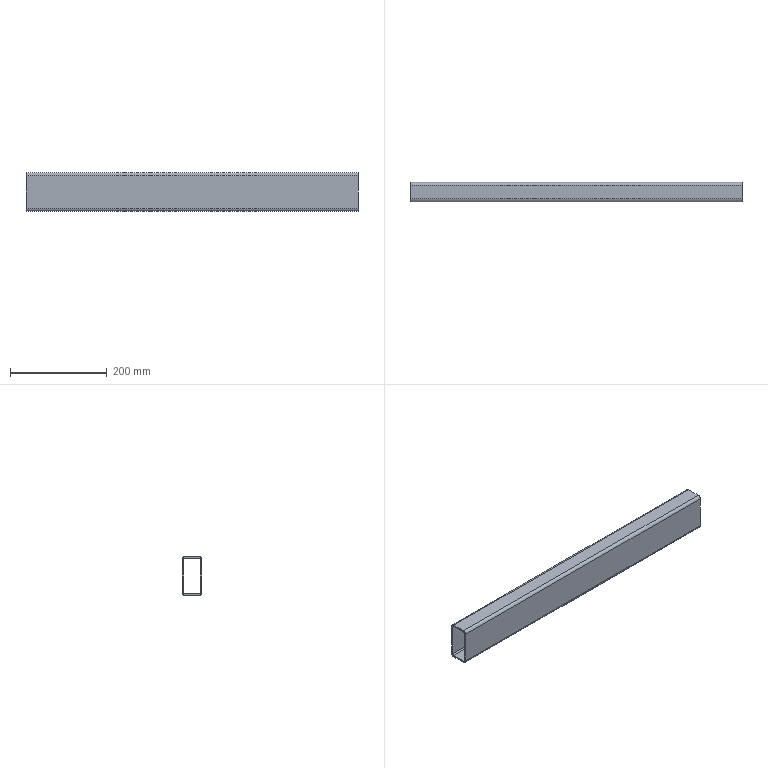Part | 1 solid | 34 faces | box 686 x 40 x 80 mm | volume 451963 mm3 | cylinder 24 | plane 10 | commonest cylinder face diameters 8.5 x16 6 x4 12 x4
STEP:
#1=CARTESIAN_POINT('',(478.,17.,13.25));
#2=VERTEX_POINT('',#1);
#3=CARTESIAN_POINT('',(478.,17.,21.75));
#4=VERTEX_POINT('',#3);
#5=CARTESIAN_POINT('',(478.,17.,17.5));
#6=DIRECTION('',(0.,1.,0.));
#7=DIRECTION('',(0.,0.,-1.));
#8=AXIS2_PLACEMENT_3D('',#5,#6,#7);
#9=CIRCLE('',#8,4.25);
#10=EDGE_CURVE('',#2,#4,#9,.T.);
#11=ORIENTED_EDGE('',*,*,#10,.F.);
#12=CARTESIAN_POINT('',(478.,20.,13.25));
#13=VERTEX_POINT('',#12);
#14=CARTESIAN_POINT('',(478.,-20.001,13.25));
#15=DIRECTION('',(0.,1.,0.));
#16=VECTOR('',#15,1000.);
#17=LINE('',#14,#16);
#18=EDGE_CURVE('',#2,#13,#17,.T.);
#19=ORIENTED_EDGE('',*,*,#18,.T.);
#20=CARTESIAN_POINT('',(478.,20.,21.75));
#21=VERTEX_POINT('',#20);
#22=CARTESIAN_POINT('',(478.,20.,17.5));
#23=DIRECTION('',(0.,1.,0.));
#24=DIRECTION('',(0.,0.,-1.));
#25=AXIS2_PLACEMENT_3D('',#22,#23,#24);
#26=CIRCLE('',#25,4.25);
#27=EDGE_CURVE('',#13,#21,#26,.T.);
#28=ORIENTED_EDGE('',*,*,#27,.T.);
#29=CARTESIAN_POINT('',(478.,-20.001,21.75));
#30=DIRECTION('',(0.,1.,0.));
#31=VECTOR('',#30,1000.);
#32=LINE('',#29,#31);
#33=EDGE_CURVE('',#4,#21,#32,.T.);
#34=ORIENTED_EDGE('',*,*,#33,.F.);
#35=EDGE_LOOP('',(#11,#19,#28,#34));
#36=FACE_OUTER_BOUND('',#35,.T.);
#37=CARTESIAN_POINT('',(478.,-20.001,17.5));
#38=DIRECTION('',(0.,1.,0.));
#39=DIRECTION('',(0.,0.,1.));
#40=AXIS2_PLACEMENT_3D('',#37,#38,#39);
#41=CYLINDRICAL_SURFACE('',#40,4.25);
#42=ADVANCED_FACE('',(#36),#41,.F.);
#43=CARTESIAN_POINT('',(208.,17.,13.25));
#44=VERTEX_POINT('',#43);
#45=CARTESIAN_POINT('',(208.,17.,21.75));
#46=VERTEX_POINT('',#45);
#47=CARTESIAN_POINT('',(208.,17.,17.5));
#48=DIRECTION('',(0.,1.,0.));
#49=DIRECTION('',(0.,0.,-1.));
#50=AXIS2_PLACEMENT_3D('',#47,#48,#49);
#51=CIRCLE('',#50,4.25);
#52=EDGE_CURVE('',#44,#46,#51,.T.);
#53=ORIENTED_EDGE('',*,*,#52,.F.);
#54=CARTESIAN_POINT('',(208.,20.,13.25));
#55=VERTEX_POINT('',#54);
#56=CARTESIAN_POINT('',(208.,-20.001,13.25));
#57=DIRECTION('',(0.,1.,0.));
#58=VECTOR('',#57,1000.);
#59=LINE('',#56,#58);
#60=EDGE_CURVE('',#44,#55,#59,.T.);
#61=ORIENTED_EDGE('',*,*,#60,.T.);
#62=CARTESIAN_POINT('',(208.,20.,21.75));
#63=VERTEX_POINT('',#62);
#64=CARTESIAN_POINT('',(208.,20.,17.5));
#65=DIRECTION('',(0.,1.,0.));
#66=DIRECTION('',(0.,0.,1.));
#67=AXIS2_PLACEMENT_3D('',#64,#65,#66);
#68=CIRCLE('',#67,4.25);
#69=EDGE_CURVE('',#55,#63,#68,.T.);
#70=ORIENTED_EDGE('',*,*,#69,.T.);
#71=CARTESIAN_POINT('',(208.,-20.001,21.75));
#72=DIRECTION('',(0.,1.,0.));
#73=VECTOR('',#72,1000.);
#74=LINE('',#71,#73);
#75=EDGE_CURVE('',#46,#63,#74,.T.);
#76=ORIENTED_EDGE('',*,*,#75,.F.);
#77=EDGE_LOOP('',(#53,#61,#70,#76));
#78=FACE_OUTER_BOUND('',#77,.T.);
#79=CARTESIAN_POINT('',(208.,-20.001,17.5));
#80=DIRECTION('',(0.,1.,0.));
#81=DIRECTION('',(0.,0.,1.));
#82=AXIS2_PLACEMENT_3D('',#79,#80,#81);
#83=CYLINDRICAL_SURFACE('',#82,4.25);
#84=ADVANCED_FACE('',(#78),#83,.F.);
#85=CARTESIAN_POINT('',(158.,17.,13.25));
#86=VERTEX_POINT('',#85);
#87=CARTESIAN_POINT('',(158.,17.,21.75));
#88=VERTEX_POINT('',#87);
#89=CARTESIAN_POINT('',(158.,17.,17.5));
#90=DIRECTION('',(0.,1.,0.));
#91=DIRECTION('',(0.,0.,-1.));
#92=AXIS2_PLACEMENT_3D('',#89,#90,#91);
#93=CIRCLE('',#92,4.25);
#94=EDGE_CURVE('',#86,#88,#93,.T.);
#95=ORIENTED_EDGE('',*,*,#94,.F.);
#96=CARTESIAN_POINT('',(158.,20.,13.25));
#97=VERTEX_POINT('',#96);
#98=CARTESIAN_POINT('',(158.,-20.001,13.25));
#99=DIRECTION('',(0.,1.,0.));
#100=VECTOR('',#99,1000.);
#101=LINE('',#98,#100);
#102=EDGE_CURVE('',#86,#97,#101,.T.);
#103=ORIENTED_EDGE('',*,*,#102,.T.);
#104=CARTESIAN_POINT('',(158.,20.,21.75));
#105=VERTEX_POINT('',#104);
#106=CARTESIAN_POINT('',(158.,20.,17.5));
#107=DIRECTION('',(0.,1.,0.));
#108=DIRECTION('',(0.,0.,1.));
#109=AXIS2_PLACEMENT_3D('',#106,#107,#108);
#110=CIRCLE('',#109,4.25);
#111=EDGE_CURVE('',#97,#105,#110,.T.);
#112=ORIENTED_EDGE('',*,*,#111,.T.);
#113=CARTESIAN_POINT('',(158.,-20.001,21.75));
#114=DIRECTION('',(0.,1.,0.));
#115=VECTOR('',#114,1000.);
#116=LINE('',#113,#115);
#117=EDGE_CURVE('',#88,#105,#116,.T.);
#118=ORIENTED_EDGE('',*,*,#117,.F.);
#119=EDGE_LOOP('',(#95,#103,#112,#118));
#120=FACE_OUTER_BOUND('',#119,.T.);
#121=CARTESIAN_POINT('',(158.,-20.001,17.5));
#122=DIRECTION('',(0.,1.,0.));
#123=DIRECTION('',(0.,0.,1.));
#124=AXIS2_PLACEMENT_3D('',#121,#122,#123);
#125=CYLINDRICAL_SURFACE('',#124,4.25);
#126=ADVANCED_FACE('',(#120),#125,.F.);
#127=CARTESIAN_POINT('',(208.,17.,-21.75));
#128=VERTEX_POINT('',#127);
#129=CARTESIAN_POINT('',(208.,17.,-13.25));
#130=VERTEX_POINT('',#129);
#131=CARTESIAN_POINT('',(208.,17.,-17.5));
#132=DIRECTION('',(0.,1.,0.));
#133=DIRECTION('',(0.,0.,-1.));
#134=AXIS2_PLACEMENT_3D('',#131,#132,#133);
#135=CIRCLE('',#134,4.25);
#136=EDGE_CURVE('',#128,#130,#135,.T.);
#137=ORIENTED_EDGE('',*,*,#136,.F.);
#138=CARTESIAN_POINT('',(208.,20.,-21.75));
#139=VERTEX_POINT('',#138);
#140=CARTESIAN_POINT('',(208.,-20.001,-21.75));
#141=DIRECTION('',(0.,1.,0.));
#142=VECTOR('',#141,1000.);
#143=LINE('',#140,#142);
#144=EDGE_CURVE('',#128,#139,#143,.T.);
#145=ORIENTED_EDGE('',*,*,#144,.T.);
#146=CARTESIAN_POINT('',(208.,20.,-13.25));
#147=VERTEX_POINT('',#146);
#148=CARTESIAN_POINT('',(208.,20.,-17.5));
#149=DIRECTION('',(0.,1.,0.));
#150=DIRECTION('',(0.,0.,1.));
#151=AXIS2_PLACEMENT_3D('',#148,#149,#150);
#152=CIRCLE('',#151,4.25);
#153=EDGE_CURVE('',#139,#147,#152,.T.);
#154=ORIENTED_EDGE('',*,*,#153,.T.);
#155=CARTESIAN_POINT('',(208.,-20.001,-13.25));
#156=DIRECTION('',(0.,1.,0.));
#157=VECTOR('',#156,1000.);
#158=LINE('',#155,#157);
#159=EDGE_CURVE('',#130,#147,#158,.T.);
#160=ORIENTED_EDGE('',*,*,#159,.F.);
#161=EDGE_LOOP('',(#137,#145,#154,#160));
#162=FACE_OUTER_BOUND('',#161,.T.);
#163=CARTESIAN_POINT('',(208.,-20.001,-17.5));
#164=DIRECTION('',(0.,1.,0.));
#165=DIRECTION('',(0.,0.,1.));
#166=AXIS2_PLACEMENT_3D('',#163,#164,#165);
#167=CYLINDRICAL_SURFACE('',#166,4.25);
#168=ADVANCED_FACE('',(#162),#167,.F.);
#169=CARTESIAN_POINT('',(528.,17.,-21.75));
#170=VERTEX_POINT('',#169);
#171=CARTESIAN_POINT('',(528.,17.,-13.25));
#172=VERTEX_POINT('',#171);
#173=CARTESIAN_POINT('',(528.,17.,-17.5));
#174=DIRECTION('',(0.,1.,0.));
#175=DIRECTION('',(0.,0.,-1.));
#176=AXIS2_PLACEMENT_3D('',#173,#174,#175);
#177=CIRCLE('',#176,4.25);
#178=EDGE_CURVE('',#170,#172,#177,.T.);
#179=ORIENTED_EDGE('',*,*,#178,.F.);
#180=CARTESIAN_POINT('',(528.,20.,-21.75));
#181=VERTEX_POINT('',#180);
#182=CARTESIAN_POINT('',(528.,-20.001,-21.75));
#183=DIRECTION('',(0.,1.,0.));
#184=VECTOR('',#183,1000.);
#185=LINE('',#182,#184);
#186=EDGE_CURVE('',#170,#181,#185,.T.);
#187=ORIENTED_EDGE('',*,*,#186,.T.);
#188=CARTESIAN_POINT('',(528.,20.,-13.25));
#189=VERTEX_POINT('',#188);
#190=CARTESIAN_POINT('',(528.,20.,-17.5));
#191=DIRECTION('',(0.,1.,0.));
#192=DIRECTION('',(0.,0.,-1.));
#193=AXIS2_PLACEMENT_3D('',#190,#191,#192);
#194=CIRCLE('',#193,4.25);
#195=EDGE_CURVE('',#181,#189,#194,.T.);
#196=ORIENTED_EDGE('',*,*,#195,.T.);
#197=CARTESIAN_POINT('',(528.,-20.001,-13.25));
#198=DIRECTION('',(0.,1.,0.));
#199=VECTOR('',#198,1000.);
#200=LINE('',#197,#199);
#201=EDGE_CURVE('',#172,#189,#200,.T.);
#202=ORIENTED_EDGE('',*,*,#201,.F.);
#203=EDGE_LOOP('',(#179,#187,#196,#202));
#204=FACE_OUTER_BOUND('',#203,.T.);
#205=CARTESIAN_POINT('',(528.,-20.001,-17.5));
#206=DIRECTION('',(0.,1.,0.));
#207=DIRECTION('',(0.,0.,1.));
#208=AXIS2_PLACEMENT_3D('',#205,#206,#207);
#209=CYLINDRICAL_SURFACE('',#208,4.25);
#210=ADVANCED_FACE('',(#204),#209,.F.);
#211=CARTESIAN_POINT('',(478.,17.,-21.75));
#212=VERTEX_POINT('',#211);
#213=CARTESIAN_POINT('',(478.,17.,-13.25));
#214=VERTEX_POINT('',#213);
#215=CARTESIAN_POINT('',(478.,17.,-17.5));
#216=DIRECTION('',(0.,1.,0.));
#217=DIRECTION('',(0.,0.,-1.));
#218=AXIS2_PLACEMENT_3D('',#215,#216,#217);
#219=CIRCLE('',#218,4.25);
#220=EDGE_CURVE('',#212,#214,#219,.T.);
#221=ORIENTED_EDGE('',*,*,#220,.F.);
#222=CARTESIAN_POINT('',(478.,20.,-21.75));
#223=VERTEX_POINT('',#222);
#224=CARTESIAN_POINT('',(478.,-20.001,-21.75));
#225=DIRECTION('',(0.,1.,0.));
#226=VECTOR('',#225,1000.);
#227=LINE('',#224,#226);
#228=EDGE_CURVE('',#212,#223,#227,.T.);
#229=ORIENTED_EDGE('',*,*,#228,.T.);
#230=CARTESIAN_POINT('',(478.,20.,-13.25));
#231=VERTEX_POINT('',#230);
#232=CARTESIAN_POINT('',(478.,20.,-17.5));
#233=DIRECTION('',(0.,1.,0.));
#234=DIRECTION('',(0.,0.,-1.));
#235=AXIS2_PLACEMENT_3D('',#232,#233,#234);
#236=CIRCLE('',#235,4.25);
#237=EDGE_CURVE('',#223,#231,#236,.T.);
#238=ORIENTED_EDGE('',*,*,#237,.T.);
#239=CARTESIAN_POINT('',(478.,-20.001,-13.25));
#240=DIRECTION('',(0.,1.,0.));
#241=VECTOR('',#240,1000.);
#242=LINE('',#239,#241);
#243=EDGE_CURVE('',#214,#231,#242,.T.);
#244=ORIENTED_EDGE('',*,*,#243,.F.);
#245=EDGE_LOOP('',(#221,#229,#238,#244));
#246=FACE_OUTER_BOUND('',#245,.T.);
#247=CARTESIAN_POINT('',(478.,-20.001,-17.5));
#248=DIRECTION('',(0.,1.,0.));
#249=DIRECTION('',(0.,0.,1.));
#250=AXIS2_PLACEMENT_3D('',#247,#248,#249);
#251=CYLINDRICAL_SURFACE('',#250,4.25);
#252=ADVANCED_FACE('',(#246),#251,.F.);
#253=CARTESIAN_POINT('',(528.,17.,13.25));
#254=VERTEX_POINT('',#253);
#255=CARTESIAN_POINT('',(528.,17.,21.75));
#256=VERTEX_POINT('',#255);
#257=CARTESIAN_POINT('',(528.,17.,17.5));
#258=DIRECTION('',(0.,1.,0.));
#259=DIRECTION('',(0.,0.,-1.));
#260=AXIS2_PLACEMENT_3D('',#257,#258,#259);
#261=CIRCLE('',#260,4.25);
#262=EDGE_CURVE('',#254,#256,#261,.T.);
#263=ORIENTED_EDGE('',*,*,#262,.F.);
#264=CARTESIAN_POINT('',(528.,20.,13.25));
#265=VERTEX_POINT('',#264);
#266=CARTESIAN_POINT('',(528.,-20.001,13.25));
#267=DIRECTION('',(0.,1.,0.));
#268=VECTOR('',#267,1000.);
#269=LINE('',#266,#268);
#270=EDGE_CURVE('',#254,#265,#269,.T.);
#271=ORIENTED_EDGE('',*,*,#270,.T.);
#272=CARTESIAN_POINT('',(528.,20.,21.75));
#273=VERTEX_POINT('',#272);
#274=CARTESIAN_POINT('',(528.,20.,17.5));
#275=DIRECTION('',(0.,1.,0.));
#276=DIRECTION('',(0.,0.,-1.));
#277=AXIS2_PLACEMENT_3D('',#274,#275,#276);
#278=CIRCLE('',#277,4.25);
#279=EDGE_CURVE('',#265,#273,#278,.T.);
#280=ORIENTED_EDGE('',*,*,#279,.T.);
#281=CARTESIAN_POINT('',(528.,-20.001,21.75));
#282=DIRECTION('',(0.,1.,0.));
#283=VECTOR('',#282,1000.);
#284=LINE('',#281,#283);
#285=EDGE_CURVE('',#256,#273,#284,.T.);
#286=ORIENTED_EDGE('',*,*,#285,.F.);
#287=EDGE_LOOP('',(#263,#271,#280,#286));
#288=FACE_OUTER_BOUND('',#287,.T.);
#289=CARTESIAN_POINT('',(528.,-20.001,17.5));
#290=DIRECTION('',(0.,1.,0.));
#291=DIRECTION('',(0.,0.,1.));
#292=AXIS2_PLACEMENT_3D('',#289,#290,#291);
#293=CYLINDRICAL_SURFACE('',#292,4.25);
#294=ADVANCED_FACE('',(#288),#293,.F.);
#295=CARTESIAN_POINT('',(158.,17.,-21.75));
#296=VERTEX_POINT('',#295);
#297=CARTESIAN_POINT('',(158.,17.,-13.25));
#298=VERTEX_POINT('',#297);
#299=CARTESIAN_POINT('',(158.,17.,-17.5));
#300=DIRECTION('',(0.,1.,0.));
#301=DIRECTION('',(0.,0.,-1.));
#302=AXIS2_PLACEMENT_3D('',#299,#300,#301);
#303=CIRCLE('',#302,4.25);
#304=EDGE_CURVE('',#296,#298,#303,.T.);
#305=ORIENTED_EDGE('',*,*,#304,.F.);
#306=CARTESIAN_POINT('',(158.,20.,-21.75));
#307=VERTEX_POINT('',#306);
#308=CARTESIAN_POINT('',(158.,-20.001,-21.75));
#309=DIRECTION('',(0.,1.,0.));
#310=VECTOR('',#309,1000.);
#311=LINE('',#308,#310);
#312=EDGE_CURVE('',#296,#307,#311,.T.);
#313=ORIENTED_EDGE('',*,*,#312,.T.);
#314=CARTESIAN_POINT('',(158.,20.,-13.25));
#315=VERTEX_POINT('',#314);
#316=CARTESIAN_POINT('',(158.,20.,-17.5));
#317=DIRECTION('',(0.,1.,0.));
#318=DIRECTION('',(0.,0.,1.));
#319=AXIS2_PLACEMENT_3D('',#316,#317,#318);
#320=CIRCLE('',#319,4.25);
#321=EDGE_CURVE('',#307,#315,#320,.T.);
#322=ORIENTED_EDGE('',*,*,#321,.T.);
#323=CARTESIAN_POINT('',(158.,-20.001,-13.25));
#324=DIRECTION('',(0.,1.,0.));
#325=VECTOR('',#324,1000.);
#326=LINE('',#323,#325);
#327=EDGE_CURVE('',#298,#315,#326,.T.);
#328=ORIENTED_EDGE('',*,*,#327,.F.);
#329=EDGE_LOOP('',(#305,#313,#322,#328));
#330=FACE_OUTER_BOUND('',#329,.T.);
#331=CARTESIAN_POINT('',(158.,-20.001,-17.5));
#332=DIRECTION('',(0.,1.,0.));
#333=DIRECTION('',(0.,0.,1.));
#334=AXIS2_PLACEMENT_3D('',#331,#332,#333);
#335=CYLINDRICAL_SURFACE('',#334,4.25);
#336=ADVANCED_FACE('',(#330),#335,.F.);
#337=CARTESIAN_POINT('',(0.,20.,34.));
#338=VERTEX_POINT('',#337);
#339=CARTESIAN_POINT('',(0.,14.,40.));
#340=VERTEX_POINT('',#339);
#341=CARTESIAN_POINT('',(0.,14.,34.));
#342=DIRECTION('',(1.,0.,0.));
#343=DIRECTION('',(0.,0.,-1.));
#344=AXIS2_PLACEMENT_3D('',#341,#342,#343);
#345=CIRCLE('',#344,6.);
#346=EDGE_CURVE('',#338,#340,#345,.T.);
#347=ORIENTED_EDGE('',*,*,#346,.T.);
#348=CARTESIAN_POINT('',(686.,14.,40.));
#349=VERTEX_POINT('',#348);
#350=CARTESIAN_POINT('',(686.,14.,40.));
#351=DIRECTION('',(-1.,0.,0.));
#352=VECTOR('',#351,1000.);
#353=LINE('',#350,#352);
#354=EDGE_CURVE('',#349,#340,#353,.T.);
#355=ORIENTED_EDGE('',*,*,#354,.F.);
#356=CARTESIAN_POINT('',(686.,20.,34.));
#357=VERTEX_POINT('',#356);
#358=CARTESIAN_POINT('',(686.,14.,34.));
#359=DIRECTION('',(1.,0.,0.));
#360=DIRECTION('',(0.,0.,-1.));
#361=AXIS2_PLACEMENT_3D('',#358,#359,#360);
#362=CIRCLE('',#361,6.);
#363=EDGE_CURVE('',#357,#349,#362,.T.);
#364=ORIENTED_EDGE('',*,*,#363,.F.);
#365=CARTESIAN_POINT('',(686.,20.,34.));
#366=DIRECTION('',(-1.,0.,0.));
#367=VECTOR('',#366,1000.);
#368=LINE('',#365,#367);
#369=EDGE_CURVE('',#357,#338,#368,.T.);
#370=ORIENTED_EDGE('',*,*,#369,.T.);
#371=EDGE_LOOP('',(#347,#355,#364,#370));
#372=FACE_OUTER_BOUND('',#371,.T.);
#373=CARTESIAN_POINT('',(686.,14.,34.));
#374=DIRECTION('',(-1.,0.,0.));
#375=DIRECTION('',(0.,0.,1.));
#376=AXIS2_PLACEMENT_3D('',#373,#374,#375);
#377=CYLINDRICAL_SURFACE('',#376,6.);
#378=ADVANCED_FACE('',(#372),#377,.T.);
#379=CARTESIAN_POINT('',(0.,-14.,40.));
#380=VERTEX_POINT('',#379);
#381=CARTESIAN_POINT('',(0.,14.,40.));
#382=DIRECTION('',(0.,-1.,0.));
#383=VECTOR('',#382,1000.);
#384=LINE('',#381,#383);
#385=EDGE_CURVE('',#340,#380,#384,.T.);
#386=ORIENTED_EDGE('',*,*,#385,.T.);
#387=CARTESIAN_POINT('',(686.,-14.,40.));
#388=VERTEX_POINT('',#387);
#389=CARTESIAN_POINT('',(686.,-14.,40.));
#390=DIRECTION('',(-1.,0.,0.));
#391=VECTOR('',#390,1000.);
#392=LINE('',#389,#391);
#393=EDGE_CURVE('',#388,#380,#392,.T.);
#394=ORIENTED_EDGE('',*,*,#393,.F.);
#395=CARTESIAN_POINT('',(686.,14.,40.));
#396=DIRECTION('',(0.,-1.,0.));
#397=VECTOR('',#396,1000.);
#398=LINE('',#395,#397);
#399=EDGE_CURVE('',#349,#388,#398,.T.);
#400=ORIENTED_EDGE('',*,*,#399,.F.);
#401=ORIENTED_EDGE('',*,*,#354,.T.);
#402=EDGE_LOOP('',(#386,#394,#400,#401));
#403=FACE_OUTER_BOUND('',#402,.T.);
#404=CARTESIAN_POINT('',(686.,14.,40.));
#405=DIRECTION('',(0.,0.,-1.));
#406=DIRECTION('',(-1.,0.,0.));
#407=AXIS2_PLACEMENT_3D('',#404,#405,#406);
#408=PLANE('',#407);
#409=ADVANCED_FACE('',(#403),#408,.F.);
#410=CARTESIAN_POINT('',(0.,-20.,34.));
#411=VERTEX_POINT('',#410);
#412=CARTESIAN_POINT('',(0.,-14.,34.));
#413=DIRECTION('',(1.,0.,0.));
#414=DIRECTION('',(0.,0.,-1.));
#415=AXIS2_PLACEMENT_3D('',#412,#413,#414);
#416=CIRCLE('',#415,6.);
#417=EDGE_CURVE('',#380,#411,#416,.T.);
#418=ORIENTED_EDGE('',*,*,#417,.T.);
#419=CARTESIAN_POINT('',(686.,-20.,34.));
#420=VERTEX_POINT('',#419);
#421=CARTESIAN_POINT('',(686.,-20.,34.));
#422=DIRECTION('',(-1.,0.,0.));
#423=VECTOR('',#422,1000.);
#424=LINE('',#421,#423);
#425=EDGE_CURVE('',#420,#411,#424,.T.);
#426=ORIENTED_EDGE('',*,*,#425,.F.);
#427=CARTESIAN_POINT('',(686.,-14.,34.));
#428=DIRECTION('',(1.,0.,0.));
#429=DIRECTION('',(0.,0.,-1.));
#430=AXIS2_PLACEMENT_3D('',#427,#428,#429);
#431=CIRCLE('',#430,6.);
#432=EDGE_CURVE('',#388,#420,#431,.T.);
#433=ORIENTED_EDGE('',*,*,#432,.F.);
#434=ORIENTED_EDGE('',*,*,#393,.T.);
#435=EDGE_LOOP('',(#418,#426,#433,#434));
#436=FACE_OUTER_BOUND('',#435,.T.);
#437=CARTESIAN_POINT('',(686.,-14.,34.));
#438=DIRECTION('',(-1.,0.,0.));
#439=DIRECTION('',(0.,0.,1.));
#440=AXIS2_PLACEMENT_3D('',#437,#438,#439);
#441=CYLINDRICAL_SURFACE('',#440,6.);
#442=ADVANCED_FACE('',(#436),#441,.T.);
#443=CARTESIAN_POINT('',(0.,-20.,-34.));
#444=VERTEX_POINT('',#443);
#445=CARTESIAN_POINT('',(0.,-20.,-34.));
#446=DIRECTION('',(0.,0.,-1.));
#447=VECTOR('',#446,1000.);
#448=LINE('',#445,#447);
#449=EDGE_CURVE('',#411,#444,#448,.T.);
#450=ORIENTED_EDGE('',*,*,#449,.T.);
#451=CARTESIAN_POINT('',(686.,-20.,-34.));
#452=VERTEX_POINT('',#451);
#453=CARTESIAN_POINT('',(686.,-20.,-34.));
#454=DIRECTION('',(-1.,0.,0.));
#455=VECTOR('',#454,1000.);
#456=LINE('',#453,#455);
#457=EDGE_CURVE('',#452,#444,#456,.T.);
#458=ORIENTED_EDGE('',*,*,#457,.F.);
#459=CARTESIAN_POINT('',(686.,-20.,-34.));
#460=DIRECTION('',(0.,0.,-1.));
#461=VECTOR('',#460,1000.);
#462=LINE('',#459,#461);
#463=EDGE_CURVE('',#420,#452,#462,.T.);
#464=ORIENTED_EDGE('',*,*,#463,.F.);
#465=ORIENTED_EDGE('',*,*,#425,.T.);
#466=EDGE_LOOP('',(#450,#458,#464,#465));
#467=FACE_OUTER_BOUND('',#466,.T.);
#468=CARTESIAN_POINT('',(686.,-20.,-34.));
#469=DIRECTION('',(0.,1.,0.));
#470=DIRECTION('',(0.,0.,1.));
#471=AXIS2_PLACEMENT_3D('',#468,#469,#470);
#472=PLANE('',#471);
#473=ADVANCED_FACE('',(#467),#472,.F.);
#474=CARTESIAN_POINT('',(0.,-14.,-40.));
#475=VERTEX_POINT('',#474);
#476=CARTESIAN_POINT('',(0.,-14.,-34.));
#477=DIRECTION('',(1.,0.,0.));
#478=DIRECTION('',(0.,0.,-1.));
#479=AXIS2_PLACEMENT_3D('',#476,#477,#478);
#480=CIRCLE('',#479,6.);
#481=EDGE_CURVE('',#444,#475,#480,.T.);
#482=ORIENTED_EDGE('',*,*,#481,.T.);
#483=CARTESIAN_POINT('',(686.,-14.,-40.));
#484=VERTEX_POINT('',#483);
#485=CARTESIAN_POINT('',(686.,-14.,-40.));
#486=DIRECTION('',(-1.,0.,0.));
#487=VECTOR('',#486,1000.);
#488=LINE('',#485,#487);
#489=EDGE_CURVE('',#484,#475,#488,.T.);
#490=ORIENTED_EDGE('',*,*,#489,.F.);
#491=CARTESIAN_POINT('',(686.,-14.,-34.));
#492=DIRECTION('',(1.,0.,0.));
#493=DIRECTION('',(0.,0.,-1.));
#494=AXIS2_PLACEMENT_3D('',#491,#492,#493);
#495=CIRCLE('',#494,6.);
#496=EDGE_CURVE('',#452,#484,#495,.T.);
#497=ORIENTED_EDGE('',*,*,#496,.F.);
#498=ORIENTED_EDGE('',*,*,#457,.T.);
#499=EDGE_LOOP('',(#482,#490,#497,#498));
#500=FACE_OUTER_BOUND('',#499,.T.);
#501=CARTESIAN_POINT('',(686.,-14.,-34.));
#502=DIRECTION('',(-1.,0.,0.));
#503=DIRECTION('',(0.,0.,1.));
#504=AXIS2_PLACEMENT_3D('',#501,#502,#503);
#505=CYLINDRICAL_SURFACE('',#504,6.);
#506=ADVANCED_FACE('',(#500),#505,.T.);
#507=CARTESIAN_POINT('',(0.,14.,-40.));
#508=VERTEX_POINT('',#507);
#509=CARTESIAN_POINT('',(0.,-14.,-40.));
#510=DIRECTION('',(0.,1.,0.));
#511=VECTOR('',#510,1000.);
#512=LINE('',#509,#511);
#513=EDGE_CURVE('',#475,#508,#512,.T.);
#514=ORIENTED_EDGE('',*,*,#513,.T.);
#515=CARTESIAN_POINT('',(686.,14.,-40.));
#516=VERTEX_POINT('',#515);
#517=CARTESIAN_POINT('',(686.,14.,-40.));
#518=DIRECTION('',(-1.,0.,0.));
#519=VECTOR('',#518,1000.);
#520=LINE('',#517,#519);
#521=EDGE_CURVE('',#516,#508,#520,.T.);
#522=ORIENTED_EDGE('',*,*,#521,.F.);
#523=CARTESIAN_POINT('',(686.,-14.,-40.));
#524=DIRECTION('',(0.,1.,0.));
#525=VECTOR('',#524,1000.);
#526=LINE('',#523,#525);
#527=EDGE_CURVE('',#484,#516,#526,.T.);
#528=ORIENTED_EDGE('',*,*,#527,.F.);
#529=ORIENTED_EDGE('',*,*,#489,.T.);
#530=EDGE_LOOP('',(#514,#522,#528,#529));
#531=FACE_OUTER_BOUND('',#530,.T.);
#532=CARTESIAN_POINT('',(686.,-14.,-40.));
#533=DIRECTION('',(0.,0.,1.));
#534=DIRECTION('',(1.,0.,0.));
#535=AXIS2_PLACEMENT_3D('',#532,#533,#534);
#536=PLANE('',#535);
#537=ADVANCED_FACE('',(#531),#536,.F.);
#538=CARTESIAN_POINT('',(0.,20.,-34.));
#539=VERTEX_POINT('',#538);
#540=CARTESIAN_POINT('',(0.,14.,-34.));
#541=DIRECTION('',(1.,0.,0.));
#542=DIRECTION('',(0.,0.,-1.));
#543=AXIS2_PLACEMENT_3D('',#540,#541,#542);
#544=CIRCLE('',#543,6.);
#545=EDGE_CURVE('',#508,#539,#544,.T.);
#546=ORIENTED_EDGE('',*,*,#545,.T.);
#547=CARTESIAN_POINT('',(686.,20.,-34.));
#548=VERTEX_POINT('',#547);
#549=CARTESIAN_POINT('',(686.,20.,-34.));
#550=DIRECTION('',(-1.,0.,0.));
#551=VECTOR('',#550,1000.);
#552=LINE('',#549,#551);
#553=EDGE_CURVE('',#548,#539,#552,.T.);
#554=ORIENTED_EDGE('',*,*,#553,.F.);
#555=CARTESIAN_POINT('',(686.,14.,-34.));
#556=DIRECTION('',(1.,0.,0.));
#557=DIRECTION('',(0.,0.,-1.));
#558=AXIS2_PLACEMENT_3D('',#555,#556,#557);
#559=CIRCLE('',#558,6.);
#560=EDGE_CURVE('',#516,#548,#559,.T.);
#561=ORIENTED_EDGE('',*,*,#560,.F.);
#562=ORIENTED_EDGE('',*,*,#521,.T.);
#563=EDGE_LOOP('',(#546,#554,#561,#562));
#564=FACE_OUTER_BOUND('',#563,.T.);
#565=CARTESIAN_POINT('',(686.,14.,-34.));
#566=DIRECTION('',(-1.,0.,0.));
#567=DIRECTION('',(0.,0.,1.));
#568=AXIS2_PLACEMENT_3D('',#565,#566,#567);
#569=CYLINDRICAL_SURFACE('',#568,6.);
#570=ADVANCED_FACE('',(#564),#569,.T.);
#571=CARTESIAN_POINT('',(0.,-14.,37.));
#572=VERTEX_POINT('',#571);
#573=CARTESIAN_POINT('',(0.,-17.,34.));
#574=VERTEX_POINT('',#573);
#575=CARTESIAN_POINT('',(0.,-14.,34.));
#576=DIRECTION('',(1.,0.,0.));
#577=DIRECTION('',(0.,0.,-1.));
#578=AXIS2_PLACEMENT_3D('',#575,#576,#577);
#579=CIRCLE('',#578,3.);
#580=EDGE_CURVE('',#572,#574,#579,.T.);
#581=ORIENTED_EDGE('',*,*,#580,.F.);
#582=CARTESIAN_POINT('',(686.,-14.,37.));
#583=VERTEX_POINT('',#582);
#584=CARTESIAN_POINT('',(686.,-14.,37.));
#585=DIRECTION('',(-1.,0.,0.));
#586=VECTOR('',#585,1000.);
#587=LINE('',#584,#586);
#588=EDGE_CURVE('',#583,#572,#587,.T.);
#589=ORIENTED_EDGE('',*,*,#588,.F.);
#590=CARTESIAN_POINT('',(686.,-17.,34.));
#591=VERTEX_POINT('',#590);
#592=CARTESIAN_POINT('',(686.,-14.,34.));
#593=DIRECTION('',(1.,0.,0.));
#594=DIRECTION('',(0.,0.,-1.));
#595=AXIS2_PLACEMENT_3D('',#592,#593,#594);
#596=CIRCLE('',#595,3.);
#597=EDGE_CURVE('',#583,#591,#596,.T.);
#598=ORIENTED_EDGE('',*,*,#597,.T.);
#599=CARTESIAN_POINT('',(686.,-17.,34.));
#600=DIRECTION('',(-1.,0.,0.));
#601=VECTOR('',#600,1000.);
#602=LINE('',#599,#601);
#603=EDGE_CURVE('',#591,#574,#602,.T.);
#604=ORIENTED_EDGE('',*,*,#603,.T.);
#605=EDGE_LOOP('',(#581,#589,#598,#604));
#606=FACE_OUTER_BOUND('',#605,.T.);
#607=CARTESIAN_POINT('',(686.,-14.,34.));
#608=DIRECTION('',(-1.,0.,0.));
#609=DIRECTION('',(0.,0.,1.));
#610=AXIS2_PLACEMENT_3D('',#607,#608,#609);
#611=CYLINDRICAL_SURFACE('',#610,3.);
#612=ADVANCED_FACE('',(#606),#611,.F.);
#613=CARTESIAN_POINT('',(0.,14.,37.));
#614=VERTEX_POINT('',#613);
#615=CARTESIAN_POINT('',(0.,14.,37.));
#616=DIRECTION('',(0.,-1.,0.));
#617=VECTOR('',#616,1000.);
#618=LINE('',#615,#617);
#619=EDGE_CURVE('',#614,#572,#618,.T.);
#620=ORIENTED_EDGE('',*,*,#619,.F.);
#621=CARTESIAN_POINT('',(686.,14.,37.));
#622=VERTEX_POINT('',#621);
#623=CARTESIAN_POINT('',(686.,14.,37.));
#624=DIRECTION('',(-1.,0.,0.));
#625=VECTOR('',#624,1000.);
#626=LINE('',#623,#625);
#627=EDGE_CURVE('',#622,#614,#626,.T.);
#628=ORIENTED_EDGE('',*,*,#627,.F.);
#629=CARTESIAN_POINT('',(686.,14.,37.));
#630=DIRECTION('',(0.,-1.,0.));
#631=VECTOR('',#630,1000.);
#632=LINE('',#629,#631);
#633=EDGE_CURVE('',#622,#583,#632,.T.);
#634=ORIENTED_EDGE('',*,*,#633,.T.);
#635=ORIENTED_EDGE('',*,*,#588,.T.);
#636=EDGE_LOOP('',(#620,#628,#634,#635));
#637=FACE_OUTER_BOUND('',#636,.T.);
#638=CARTESIAN_POINT('',(686.,14.,37.));
#639=DIRECTION('',(0.,0.,-1.));
#640=DIRECTION('',(-1.,0.,0.));
#641=AXIS2_PLACEMENT_3D('',#638,#639,#640);
#642=PLANE('',#641);
#643=ADVANCED_FACE('',(#637),#642,.T.);
#644=CARTESIAN_POINT('',(0.,17.,34.));
#645=VERTEX_POINT('',#644);
#646=CARTESIAN_POINT('',(0.,14.,34.));
#647=DIRECTION('',(1.,0.,0.));
#648=DIRECTION('',(0.,0.,-1.));
#649=AXIS2_PLACEMENT_3D('',#646,#647,#648);
#650=CIRCLE('',#649,3.);
#651=EDGE_CURVE('',#645,#614,#650,.T.);
#652=ORIENTED_EDGE('',*,*,#651,.F.);
#653=CARTESIAN_POINT('',(686.,17.,34.));
#654=VERTEX_POINT('',#653);
#655=CARTESIAN_POINT('',(686.,17.,34.));
#656=DIRECTION('',(-1.,0.,0.));
#657=VECTOR('',#656,1000.);
#658=LINE('',#655,#657);
#659=EDGE_CURVE('',#654,#645,#658,.T.);
#660=ORIENTED_EDGE('',*,*,#659,.F.);
#661=CARTESIAN_POINT('',(686.,14.,34.));
#662=DIRECTION('',(1.,0.,0.));
#663=DIRECTION('',(0.,0.,-1.));
#664=AXIS2_PLACEMENT_3D('',#661,#662,#663);
#665=CIRCLE('',#664,3.);
#666=EDGE_CURVE('',#654,#622,#665,.T.);
#667=ORIENTED_EDGE('',*,*,#666,.T.);
#668=ORIENTED_EDGE('',*,*,#627,.T.);
#669=EDGE_LOOP('',(#652,#660,#667,#668));
#670=FACE_OUTER_BOUND('',#669,.T.);
#671=CARTESIAN_POINT('',(686.,14.,34.));
#672=DIRECTION('',(-1.,0.,0.));
#673=DIRECTION('',(0.,0.,1.));
#674=AXIS2_PLACEMENT_3D('',#671,#672,#673);
#675=CYLINDRICAL_SURFACE('',#674,3.);
#676=ADVANCED_FACE('',(#670),#675,.F.);
#677=CARTESIAN_POINT('',(478.,17.,17.5));
#678=DIRECTION('',(0.,1.,0.));
#679=DIRECTION('',(0.,0.,-1.));
#680=AXIS2_PLACEMENT_3D('',#677,#678,#679);
#681=CIRCLE('',#680,4.25);
#682=EDGE_CURVE('',#4,#2,#681,.T.);
#683=ORIENTED_EDGE('',*,*,#682,.T.);
#684=ORIENTED_EDGE('',*,*,#10,.T.);
#685=EDGE_LOOP('',(#683,#684));
#686=FACE_BOUND('',#685,.T.);
#687=CARTESIAN_POINT('',(208.,17.,17.5));
#688=DIRECTION('',(0.,1.,0.));
#689=DIRECTION('',(0.,0.,-1.));
#690=AXIS2_PLACEMENT_3D('',#687,#688,#689);
#691=CIRCLE('',#690,4.25);
#692=EDGE_CURVE('',#46,#44,#691,.T.);
#693=ORIENTED_EDGE('',*,*,#692,.T.);
#694=ORIENTED_EDGE('',*,*,#52,.T.);
#695=EDGE_LOOP('',(#693,#694));
#696=FACE_BOUND('',#695,.T.);
#697=CARTESIAN_POINT('',(158.,17.,17.5));
#698=DIRECTION('',(0.,1.,0.));
#699=DIRECTION('',(0.,0.,-1.));
#700=AXIS2_PLACEMENT_3D('',#697,#698,#699);
#701=CIRCLE('',#700,4.25);
#702=EDGE_CURVE('',#88,#86,#701,.T.);
#703=ORIENTED_EDGE('',*,*,#702,.T.);
#704=ORIENTED_EDGE('',*,*,#94,.T.);
#705=EDGE_LOOP('',(#703,#704));
#706=FACE_BOUND('',#705,.T.);
#707=CARTESIAN_POINT('',(208.,17.,-17.5));
#708=DIRECTION('',(0.,1.,0.));
#709=DIRECTION('',(0.,0.,-1.));
#710=AXIS2_PLACEMENT_3D('',#707,#708,#709);
#711=CIRCLE('',#710,4.25);
#712=EDGE_CURVE('',#130,#128,#711,.T.);
#713=ORIENTED_EDGE('',*,*,#712,.T.);
#714=ORIENTED_EDGE('',*,*,#136,.T.);
#715=EDGE_LOOP('',(#713,#714));
#716=FACE_BOUND('',#715,.T.);
#717=CARTESIAN_POINT('',(528.,17.,-17.5));
#718=DIRECTION('',(0.,1.,0.));
#719=DIRECTION('',(0.,0.,-1.));
#720=AXIS2_PLACEMENT_3D('',#717,#718,#719);
#721=CIRCLE('',#720,4.25);
#722=EDGE_CURVE('',#172,#170,#721,.T.);
#723=ORIENTED_EDGE('',*,*,#722,.T.);
#724=ORIENTED_EDGE('',*,*,#178,.T.);
#725=EDGE_LOOP('',(#723,#724));
#726=FACE_BOUND('',#725,.T.);
#727=CARTESIAN_POINT('',(478.,17.,-17.5));
#728=DIRECTION('',(0.,1.,0.));
#729=DIRECTION('',(0.,0.,-1.));
#730=AXIS2_PLACEMENT_3D('',#727,#728,#729);
#731=CIRCLE('',#730,4.25);
#732=EDGE_CURVE('',#214,#212,#731,.T.);
#733=ORIENTED_EDGE('',*,*,#732,.T.);
#734=ORIENTED_EDGE('',*,*,#220,.T.);
#735=EDGE_LOOP('',(#733,#734));
#736=FACE_BOUND('',#735,.T.);
#737=CARTESIAN_POINT('',(528.,17.,17.5));
#738=DIRECTION('',(0.,1.,0.));
#739=DIRECTION('',(0.,0.,-1.));
#740=AXIS2_PLACEMENT_3D('',#737,#738,#739);
#741=CIRCLE('',#740,4.25);
#742=EDGE_CURVE('',#256,#254,#741,.T.);
#743=ORIENTED_EDGE('',*,*,#742,.T.);
#744=ORIENTED_EDGE('',*,*,#262,.T.);
#745=EDGE_LOOP('',(#743,#744));
#746=FACE_BOUND('',#745,.T.);
#747=CARTESIAN_POINT('',(158.,17.,-17.5));
#748=DIRECTION('',(0.,1.,0.));
#749=DIRECTION('',(0.,0.,-1.));
#750=AXIS2_PLACEMENT_3D('',#747,#748,#749);
#751=CIRCLE('',#750,4.25);
#752=EDGE_CURVE('',#298,#296,#751,.T.);
#753=ORIENTED_EDGE('',*,*,#752,.T.);
#754=ORIENTED_EDGE('',*,*,#304,.T.);
#755=EDGE_LOOP('',(#753,#754));
#756=FACE_BOUND('',#755,.T.);
#757=CARTESIAN_POINT('',(0.,17.,-34.));
#758=VERTEX_POINT('',#757);
#759=CARTESIAN_POINT('',(0.,17.,34.));
#760=DIRECTION('',(0.,0.,1.));
#761=VECTOR('',#760,1000.);
#762=LINE('',#759,#761);
#763=EDGE_CURVE('',#758,#645,#762,.T.);
#764=ORIENTED_EDGE('',*,*,#763,.F.);
#765=CARTESIAN_POINT('',(686.,17.,-34.));
#766=VERTEX_POINT('',#765);
#767=CARTESIAN_POINT('',(686.,17.,-34.));
#768=DIRECTION('',(-1.,0.,0.));
#769=VECTOR('',#768,1000.);
#770=LINE('',#767,#769);
#771=EDGE_CURVE('',#766,#758,#770,.T.);
#772=ORIENTED_EDGE('',*,*,#771,.F.);
#773=CARTESIAN_POINT('',(686.,17.,34.));
#774=DIRECTION('',(0.,0.,1.));
#775=VECTOR('',#774,1000.);
#776=LINE('',#773,#775);
#777=EDGE_CURVE('',#766,#654,#776,.T.);
#778=ORIENTED_EDGE('',*,*,#777,.T.);
#779=ORIENTED_EDGE('',*,*,#659,.T.);
#780=EDGE_LOOP('',(#764,#772,#778,#779));
#781=FACE_OUTER_BOUND('',#780,.T.);
#782=CARTESIAN_POINT('',(686.,17.,34.));
#783=DIRECTION('',(0.,-1.,0.));
#784=DIRECTION('',(0.,0.,-1.));
#785=AXIS2_PLACEMENT_3D('',#782,#783,#784);
#786=PLANE('',#785);
#787=ADVANCED_FACE('',(#686,#696,#706,#716,#726,#736,#746,#756,#781),#786,.T.);
#788=CARTESIAN_POINT('',(0.,14.,-37.));
#789=VERTEX_POINT('',#788);
#790=CARTESIAN_POINT('',(0.,14.,-34.));
#791=DIRECTION('',(1.,0.,0.));
#792=DIRECTION('',(0.,0.,-1.));
#793=AXIS2_PLACEMENT_3D('',#790,#791,#792);
#794=CIRCLE('',#793,3.);
#795=EDGE_CURVE('',#789,#758,#794,.T.);
#796=ORIENTED_EDGE('',*,*,#795,.F.);
#797=CARTESIAN_POINT('',(686.,14.,-37.));
#798=VERTEX_POINT('',#797);
#799=CARTESIAN_POINT('',(686.,14.,-37.));
#800=DIRECTION('',(-1.,0.,0.));
#801=VECTOR('',#800,1000.);
#802=LINE('',#799,#801);
#803=EDGE_CURVE('',#798,#789,#802,.T.);
#804=ORIENTED_EDGE('',*,*,#803,.F.);
#805=CARTESIAN_POINT('',(686.,14.,-34.));
#806=DIRECTION('',(1.,0.,0.));
#807=DIRECTION('',(0.,0.,-1.));
#808=AXIS2_PLACEMENT_3D('',#805,#806,#807);
#809=CIRCLE('',#808,3.);
#810=EDGE_CURVE('',#798,#766,#809,.T.);
#811=ORIENTED_EDGE('',*,*,#810,.T.);
#812=ORIENTED_EDGE('',*,*,#771,.T.);
#813=EDGE_LOOP('',(#796,#804,#811,#812));
#814=FACE_OUTER_BOUND('',#813,.T.);
#815=CARTESIAN_POINT('',(686.,14.,-34.));
#816=DIRECTION('',(-1.,0.,0.));
#817=DIRECTION('',(0.,0.,1.));
#818=AXIS2_PLACEMENT_3D('',#815,#816,#817);
#819=CYLINDRICAL_SURFACE('',#818,3.);
#820=ADVANCED_FACE('',(#814),#819,.F.);
#821=CARTESIAN_POINT('',(0.,-14.,-37.));
#822=VERTEX_POINT('',#821);
#823=CARTESIAN_POINT('',(0.,-14.,-37.));
#824=DIRECTION('',(0.,1.,0.));
#825=VECTOR('',#824,1000.);
#826=LINE('',#823,#825);
#827=EDGE_CURVE('',#822,#789,#826,.T.);
#828=ORIENTED_EDGE('',*,*,#827,.F.);
#829=CARTESIAN_POINT('',(686.,-14.,-37.));
#830=VERTEX_POINT('',#829);
#831=CARTESIAN_POINT('',(686.,-14.,-37.));
#832=DIRECTION('',(-1.,0.,0.));
#833=VECTOR('',#832,1000.);
#834=LINE('',#831,#833);
#835=EDGE_CURVE('',#830,#822,#834,.T.);
#836=ORIENTED_EDGE('',*,*,#835,.F.);
#837=CARTESIAN_POINT('',(686.,-14.,-37.));
#838=DIRECTION('',(0.,1.,0.));
#839=VECTOR('',#838,1000.);
#840=LINE('',#837,#839);
#841=EDGE_CURVE('',#830,#798,#840,.T.);
#842=ORIENTED_EDGE('',*,*,#841,.T.);
#843=ORIENTED_EDGE('',*,*,#803,.T.);
#844=EDGE_LOOP('',(#828,#836,#842,#843));
#845=FACE_OUTER_BOUND('',#844,.T.);
#846=CARTESIAN_POINT('',(686.,-14.,-37.));
#847=DIRECTION('',(0.,0.,1.));
#848=DIRECTION('',(1.,0.,0.));
#849=AXIS2_PLACEMENT_3D('',#846,#847,#848);
#850=PLANE('',#849);
#851=ADVANCED_FACE('',(#845),#850,.T.);
#852=CARTESIAN_POINT('',(0.,-17.,-34.));
#853=VERTEX_POINT('',#852);
#854=CARTESIAN_POINT('',(0.,-14.,-34.));
#855=DIRECTION('',(1.,0.,0.));
#856=DIRECTION('',(0.,0.,-1.));
#857=AXIS2_PLACEMENT_3D('',#854,#855,#856);
#858=CIRCLE('',#857,3.);
#859=EDGE_CURVE('',#853,#822,#858,.T.);
#860=ORIENTED_EDGE('',*,*,#859,.F.);
#861=CARTESIAN_POINT('',(686.,-17.,-34.));
#862=VERTEX_POINT('',#861);
#863=CARTESIAN_POINT('',(686.,-17.,-34.));
#864=DIRECTION('',(-1.,0.,0.));
#865=VECTOR('',#864,1000.);
#866=LINE('',#863,#865);
#867=EDGE_CURVE('',#862,#853,#866,.T.);
#868=ORIENTED_EDGE('',*,*,#867,.F.);
#869=CARTESIAN_POINT('',(686.,-14.,-34.));
#870=DIRECTION('',(1.,0.,0.));
#871=DIRECTION('',(0.,0.,-1.));
#872=AXIS2_PLACEMENT_3D('',#869,#870,#871);
#873=CIRCLE('',#872,3.);
#874=EDGE_CURVE('',#862,#830,#873,.T.);
#875=ORIENTED_EDGE('',*,*,#874,.T.);
#876=ORIENTED_EDGE('',*,*,#835,.T.);
#877=EDGE_LOOP('',(#860,#868,#875,#876));
#878=FACE_OUTER_BOUND('',#877,.T.);
#879=CARTESIAN_POINT('',(686.,-14.,-34.));
#880=DIRECTION('',(-1.,0.,0.));
#881=DIRECTION('',(0.,0.,1.));
#882=AXIS2_PLACEMENT_3D('',#879,#880,#881);
#883=CYLINDRICAL_SURFACE('',#882,3.);
#884=ADVANCED_FACE('',(#878),#883,.F.);
#885=CARTESIAN_POINT('',(0.,-17.,-34.));
#886=DIRECTION('',(0.,0.,-1.));
#887=VECTOR('',#886,1000.);
#888=LINE('',#885,#887);
#889=EDGE_CURVE('',#574,#853,#888,.T.);
#890=ORIENTED_EDGE('',*,*,#889,.F.);
#891=ORIENTED_EDGE('',*,*,#603,.F.);
#892=CARTESIAN_POINT('',(686.,-17.,-34.));
#893=DIRECTION('',(0.,0.,-1.));
#894=VECTOR('',#893,1000.);
#895=LINE('',#892,#894);
#896=EDGE_CURVE('',#591,#862,#895,.T.);
#897=ORIENTED_EDGE('',*,*,#896,.T.);
#898=ORIENTED_EDGE('',*,*,#867,.T.);
#899=EDGE_LOOP('',(#890,#891,#897,#898));
#900=FACE_OUTER_BOUND('',#899,.T.);
#901=CARTESIAN_POINT('',(686.,-17.,-34.));
#902=DIRECTION('',(0.,1.,0.));
#903=DIRECTION('',(0.,0.,1.));
#904=AXIS2_PLACEMENT_3D('',#901,#902,#903);
#905=PLANE('',#904);
#906=ADVANCED_FACE('',(#900),#905,.T.);
#907=CARTESIAN_POINT('',(478.,20.,17.5));
#908=DIRECTION('',(0.,1.,0.));
#909=DIRECTION('',(0.,0.,-1.));
#910=AXIS2_PLACEMENT_3D('',#907,#908,#909);
#911=CIRCLE('',#910,4.25);
#912=EDGE_CURVE('',#21,#13,#911,.T.);
#913=ORIENTED_EDGE('',*,*,#912,.F.);
#914=ORIENTED_EDGE('',*,*,#27,.F.);
#915=EDGE_LOOP('',(#913,#914));
#916=FACE_BOUND('',#915,.T.);
#917=CARTESIAN_POINT('',(208.,20.,17.5));
#918=DIRECTION('',(0.,1.,0.));
#919=DIRECTION('',(0.,0.,1.));
#920=AXIS2_PLACEMENT_3D('',#917,#918,#919);
#921=CIRCLE('',#920,4.25);
#922=EDGE_CURVE('',#63,#55,#921,.T.);
#923=ORIENTED_EDGE('',*,*,#922,.F.);
#924=ORIENTED_EDGE('',*,*,#69,.F.);
#925=EDGE_LOOP('',(#923,#924));
#926=FACE_BOUND('',#925,.T.);
#927=CARTESIAN_POINT('',(158.,20.,17.5));
#928=DIRECTION('',(0.,1.,0.));
#929=DIRECTION('',(0.,0.,1.));
#930=AXIS2_PLACEMENT_3D('',#927,#928,#929);
#931=CIRCLE('',#930,4.25);
#932=EDGE_CURVE('',#105,#97,#931,.T.);
#933=ORIENTED_EDGE('',*,*,#932,.F.);
#934=ORIENTED_EDGE('',*,*,#111,.F.);
#935=EDGE_LOOP('',(#933,#934));
#936=FACE_BOUND('',#935,.T.);
#937=CARTESIAN_POINT('',(208.,20.,-17.5));
#938=DIRECTION('',(0.,1.,0.));
#939=DIRECTION('',(0.,0.,1.));
#940=AXIS2_PLACEMENT_3D('',#937,#938,#939);
#941=CIRCLE('',#940,4.25);
#942=EDGE_CURVE('',#147,#139,#941,.T.);
#943=ORIENTED_EDGE('',*,*,#942,.F.);
#944=ORIENTED_EDGE('',*,*,#153,.F.);
#945=EDGE_LOOP('',(#943,#944));
#946=FACE_BOUND('',#945,.T.);
#947=CARTESIAN_POINT('',(528.,20.,-17.5));
#948=DIRECTION('',(0.,1.,0.));
#949=DIRECTION('',(0.,0.,-1.));
#950=AXIS2_PLACEMENT_3D('',#947,#948,#949);
#951=CIRCLE('',#950,4.25);
#952=EDGE_CURVE('',#189,#181,#951,.T.);
#953=ORIENTED_EDGE('',*,*,#952,.F.);
#954=ORIENTED_EDGE('',*,*,#195,.F.);
#955=EDGE_LOOP('',(#953,#954));
#956=FACE_BOUND('',#955,.T.);
#957=CARTESIAN_POINT('',(478.,20.,-17.5));
#958=DIRECTION('',(0.,1.,0.));
#959=DIRECTION('',(0.,0.,-1.));
#960=AXIS2_PLACEMENT_3D('',#957,#958,#959);
#961=CIRCLE('',#960,4.25);
#962=EDGE_CURVE('',#231,#223,#961,.T.);
#963=ORIENTED_EDGE('',*,*,#962,.F.);
#964=ORIENTED_EDGE('',*,*,#237,.F.);
#965=EDGE_LOOP('',(#963,#964));
#966=FACE_BOUND('',#965,.T.);
#967=CARTESIAN_POINT('',(528.,20.,17.5));
#968=DIRECTION('',(0.,1.,0.));
#969=DIRECTION('',(0.,0.,-1.));
#970=AXIS2_PLACEMENT_3D('',#967,#968,#969);
#971=CIRCLE('',#970,4.25);
#972=EDGE_CURVE('',#273,#265,#971,.T.);
#973=ORIENTED_EDGE('',*,*,#972,.F.);
#974=ORIENTED_EDGE('',*,*,#279,.F.);
#975=EDGE_LOOP('',(#973,#974));
#976=FACE_BOUND('',#975,.T.);
#977=CARTESIAN_POINT('',(158.,20.,-17.5));
#978=DIRECTION('',(0.,1.,0.));
#979=DIRECTION('',(0.,0.,1.));
#980=AXIS2_PLACEMENT_3D('',#977,#978,#979);
#981=CIRCLE('',#980,4.25);
#982=EDGE_CURVE('',#315,#307,#981,.T.);
#983=ORIENTED_EDGE('',*,*,#982,.F.);
#984=ORIENTED_EDGE('',*,*,#321,.F.);
#985=EDGE_LOOP('',(#983,#984));
#986=FACE_BOUND('',#985,.T.);
#987=CARTESIAN_POINT('',(0.,20.,34.));
#988=DIRECTION('',(0.,0.,1.));
#989=VECTOR('',#988,1000.);
#990=LINE('',#987,#989);
#991=EDGE_CURVE('',#539,#338,#990,.T.);
#992=ORIENTED_EDGE('',*,*,#991,.T.);
#993=ORIENTED_EDGE('',*,*,#369,.F.);
#994=CARTESIAN_POINT('',(686.,20.,34.));
#995=DIRECTION('',(0.,0.,1.));
#996=VECTOR('',#995,1000.);
#997=LINE('',#994,#996);
#998=EDGE_CURVE('',#548,#357,#997,.T.);
#999=ORIENTED_EDGE('',*,*,#998,.F.);
#1000=ORIENTED_EDGE('',*,*,#553,.T.);
#1001=EDGE_LOOP('',(#992,#993,#999,#1000));
#1002=FACE_OUTER_BOUND('',#1001,.T.);
#1003=CARTESIAN_POINT('',(686.,20.,34.));
#1004=DIRECTION('',(0.,-1.,0.));
#1005=DIRECTION('',(0.,0.,-1.));
#1006=AXIS2_PLACEMENT_3D('',#1003,#1004,#1005);
#1007=PLANE('',#1006);
#1008=ADVANCED_FACE('',(#916,#926,#936,#946,#956,#966,#976,#986,#1002),#1007,.F.);
#1009=ORIENTED_EDGE('',*,*,#597,.F.);
#1010=ORIENTED_EDGE('',*,*,#633,.F.);
#1011=ORIENTED_EDGE('',*,*,#666,.F.);
#1012=ORIENTED_EDGE('',*,*,#777,.F.);
#1013=ORIENTED_EDGE('',*,*,#810,.F.);
#1014=ORIENTED_EDGE('',*,*,#841,.F.);
#1015=ORIENTED_EDGE('',*,*,#874,.F.);
#1016=ORIENTED_EDGE('',*,*,#896,.F.);
#1017=EDGE_LOOP('',(#1009,#1010,#1011,#1012,#1013,#1014,#1015,#1016));
#1018=FACE_BOUND('',#1017,.T.);
#1019=ORIENTED_EDGE('',*,*,#363,.T.);
#1020=ORIENTED_EDGE('',*,*,#399,.T.);
#1021=ORIENTED_EDGE('',*,*,#432,.T.);
#1022=ORIENTED_EDGE('',*,*,#463,.T.);
#1023=ORIENTED_EDGE('',*,*,#496,.T.);
#1024=ORIENTED_EDGE('',*,*,#527,.T.);
#1025=ORIENTED_EDGE('',*,*,#560,.T.);
#1026=ORIENTED_EDGE('',*,*,#998,.T.);
#1027=EDGE_LOOP('',(#1019,#1020,#1021,#1022,#1023,#1024,#1025,#1026));
#1028=FACE_OUTER_BOUND('',#1027,.T.);
#1029=CARTESIAN_POINT('',(686.,14.,34.));
#1030=DIRECTION('',(1.,0.,0.));
#1031=DIRECTION('',(0.,0.,-1.));
#1032=AXIS2_PLACEMENT_3D('',#1029,#1030,#1031);
#1033=PLANE('',#1032);
#1034=ADVANCED_FACE('',(#1018,#1028),#1033,.T.);
#1035=ORIENTED_EDGE('',*,*,#580,.T.);
#1036=ORIENTED_EDGE('',*,*,#889,.T.);
#1037=ORIENTED_EDGE('',*,*,#859,.T.);
#1038=ORIENTED_EDGE('',*,*,#827,.T.);
#1039=ORIENTED_EDGE('',*,*,#795,.T.);
#1040=ORIENTED_EDGE('',*,*,#763,.T.);
#1041=ORIENTED_EDGE('',*,*,#651,.T.);
#1042=ORIENTED_EDGE('',*,*,#619,.T.);
#1043=EDGE_LOOP('',(#1035,#1036,#1037,#1038,#1039,#1040,#1041,#1042));
#1044=FACE_BOUND('',#1043,.T.);
#1045=ORIENTED_EDGE('',*,*,#346,.F.);
#1046=ORIENTED_EDGE('',*,*,#991,.F.);
#1047=ORIENTED_EDGE('',*,*,#545,.F.);
#1048=ORIENTED_EDGE('',*,*,#513,.F.);
#1049=ORIENTED_EDGE('',*,*,#481,.F.);
#1050=ORIENTED_EDGE('',*,*,#449,.F.);
#1051=ORIENTED_EDGE('',*,*,#417,.F.);
#1052=ORIENTED_EDGE('',*,*,#385,.F.);
#1053=EDGE_LOOP('',(#1045,#1046,#1047,#1048,#1049,#1050,#1051,#1052));
#1054=FACE_OUTER_BOUND('',#1053,.T.);
#1055=CARTESIAN_POINT('',(0.,14.,34.));
#1056=DIRECTION('',(1.,0.,0.));
#1057=DIRECTION('',(0.,0.,-1.));
#1058=AXIS2_PLACEMENT_3D('',#1055,#1056,#1057);
#1059=PLANE('',#1058);
#1060=ADVANCED_FACE('',(#1044,#1054),#1059,.F.);
#1061=ORIENTED_EDGE('',*,*,#312,.F.);
#1062=ORIENTED_EDGE('',*,*,#752,.F.);
#1063=ORIENTED_EDGE('',*,*,#327,.T.);
#1064=ORIENTED_EDGE('',*,*,#982,.T.);
#1065=EDGE_LOOP('',(#1061,#1062,#1063,#1064));
#1066=FACE_OUTER_BOUND('',#1065,.T.);
#1067=CARTESIAN_POINT('',(158.,-20.001,-17.5));
#1068=DIRECTION('',(0.,1.,0.));
#1069=DIRECTION('',(0.,0.,1.));
#1070=AXIS2_PLACEMENT_3D('',#1067,#1068,#1069);
#1071=CYLINDRICAL_SURFACE('',#1070,4.25);
#1072=ADVANCED_FACE('',(#1066),#1071,.F.);
#1073=ORIENTED_EDGE('',*,*,#270,.F.);
#1074=ORIENTED_EDGE('',*,*,#742,.F.);
#1075=ORIENTED_EDGE('',*,*,#285,.T.);
#1076=ORIENTED_EDGE('',*,*,#972,.T.);
#1077=EDGE_LOOP('',(#1073,#1074,#1075,#1076));
#1078=FACE_OUTER_BOUND('',#1077,.T.);
#1079=CARTESIAN_POINT('',(528.,-20.001,17.5));
#1080=DIRECTION('',(0.,1.,0.));
#1081=DIRECTION('',(0.,0.,1.));
#1082=AXIS2_PLACEMENT_3D('',#1079,#1080,#1081);
#1083=CYLINDRICAL_SURFACE('',#1082,4.25);
#1084=ADVANCED_FACE('',(#1078),#1083,.F.);
#1085=ORIENTED_EDGE('',*,*,#228,.F.);
#1086=ORIENTED_EDGE('',*,*,#732,.F.);
#1087=ORIENTED_EDGE('',*,*,#243,.T.);
#1088=ORIENTED_EDGE('',*,*,#962,.T.);
#1089=EDGE_LOOP('',(#1085,#1086,#1087,#1088));
#1090=FACE_OUTER_BOUND('',#1089,.T.);
#1091=CARTESIAN_POINT('',(478.,-20.001,-17.5));
#1092=DIRECTION('',(0.,1.,0.));
#1093=DIRECTION('',(0.,0.,1.));
#1094=AXIS2_PLACEMENT_3D('',#1091,#1092,#1093);
#1095=CYLINDRICAL_SURFACE('',#1094,4.25);
#1096=ADVANCED_FACE('',(#1090),#1095,.F.);
#1097=ORIENTED_EDGE('',*,*,#186,.F.);
#1098=ORIENTED_EDGE('',*,*,#722,.F.);
#1099=ORIENTED_EDGE('',*,*,#201,.T.);
#1100=ORIENTED_EDGE('',*,*,#952,.T.);
#1101=EDGE_LOOP('',(#1097,#1098,#1099,#1100));
#1102=FACE_OUTER_BOUND('',#1101,.T.);
#1103=CARTESIAN_POINT('',(528.,-20.001,-17.5));
#1104=DIRECTION('',(0.,1.,0.));
#1105=DIRECTION('',(0.,0.,1.));
#1106=AXIS2_PLACEMENT_3D('',#1103,#1104,#1105);
#1107=CYLINDRICAL_SURFACE('',#1106,4.25);
#1108=ADVANCED_FACE('',(#1102),#1107,.F.);
#1109=ORIENTED_EDGE('',*,*,#144,.F.);
#1110=ORIENTED_EDGE('',*,*,#712,.F.);
#1111=ORIENTED_EDGE('',*,*,#159,.T.);
#1112=ORIENTED_EDGE('',*,*,#942,.T.);
#1113=EDGE_LOOP('',(#1109,#1110,#1111,#1112));
#1114=FACE_OUTER_BOUND('',#1113,.T.);
#1115=CARTESIAN_POINT('',(208.,-20.001,-17.5));
#1116=DIRECTION('',(0.,1.,0.));
#1117=DIRECTION('',(0.,0.,1.));
#1118=AXIS2_PLACEMENT_3D('',#1115,#1116,#1117);
#1119=CYLINDRICAL_SURFACE('',#1118,4.25);
#1120=ADVANCED_FACE('',(#1114),#1119,.F.);
#1121=ORIENTED_EDGE('',*,*,#102,.F.);
#1122=ORIENTED_EDGE('',*,*,#702,.F.);
#1123=ORIENTED_EDGE('',*,*,#117,.T.);
#1124=ORIENTED_EDGE('',*,*,#932,.T.);
#1125=EDGE_LOOP('',(#1121,#1122,#1123,#1124));
#1126=FACE_OUTER_BOUND('',#1125,.T.);
#1127=CARTESIAN_POINT('',(158.,-20.001,17.5));
#1128=DIRECTION('',(0.,1.,0.));
#1129=DIRECTION('',(0.,0.,1.));
#1130=AXIS2_PLACEMENT_3D('',#1127,#1128,#1129);
#1131=CYLINDRICAL_SURFACE('',#1130,4.25);
#1132=ADVANCED_FACE('',(#1126),#1131,.F.);
#1133=ORIENTED_EDGE('',*,*,#60,.F.);
#1134=ORIENTED_EDGE('',*,*,#692,.F.);
#1135=ORIENTED_EDGE('',*,*,#75,.T.);
#1136=ORIENTED_EDGE('',*,*,#922,.T.);
#1137=EDGE_LOOP('',(#1133,#1134,#1135,#1136));
#1138=FACE_OUTER_BOUND('',#1137,.T.);
#1139=CARTESIAN_POINT('',(208.,-20.001,17.5));
#1140=DIRECTION('',(0.,1.,0.));
#1141=DIRECTION('',(0.,0.,1.));
#1142=AXIS2_PLACEMENT_3D('',#1139,#1140,#1141);
#1143=CYLINDRICAL_SURFACE('',#1142,4.25);
#1144=ADVANCED_FACE('',(#1138),#1143,.F.);
#1145=ORIENTED_EDGE('',*,*,#18,.F.);
#1146=ORIENTED_EDGE('',*,*,#682,.F.);
#1147=ORIENTED_EDGE('',*,*,#33,.T.);
#1148=ORIENTED_EDGE('',*,*,#912,.T.);
#1149=EDGE_LOOP('',(#1145,#1146,#1147,#1148));
#1150=FACE_OUTER_BOUND('',#1149,.T.);
#1151=CARTESIAN_POINT('',(478.,-20.001,17.5));
#1152=DIRECTION('',(0.,1.,0.));
#1153=DIRECTION('',(0.,0.,1.));
#1154=AXIS2_PLACEMENT_3D('',#1151,#1152,#1153);
#1155=CYLINDRICAL_SURFACE('',#1154,4.25);
#1156=ADVANCED_FACE('',(#1150),#1155,.F.);
#1157=CLOSED_SHELL('',(#42,#84,#126,#168,#210,#252,#294,#336,#378,#409,#442,#473,#506,#537,#570,#612,#643,#676,#787,#820,#851,#884,#906,#1008,#1034,#1060,#1072,#1084,#1096,#1108,#1120,#1132,#1144,#1156));
#1158=MANIFOLD_SOLID_BREP('',#1157);
#1159=CARTESIAN_POINT('',(0.,0.,0.));
#1160=DIRECTION('',(0.,0.,1.));
#1161=DIRECTION('',(1.,0.,0.));
#1162=AXIS2_PLACEMENT_3D('',#1159,#1160,#1161);
#1163=(LENGTH_UNIT()NAMED_UNIT(*)SI_UNIT(.MILLI.,.METRE.));
#1164=UNCERTAINTY_MEASURE_WITH_UNIT(LENGTH_MEASURE(0.00001),#1163,'','');
#1165=(NAMED_UNIT(*)PLANE_ANGLE_UNIT()SI_UNIT($,.RADIAN.));
#1166=(NAMED_UNIT(*)SI_UNIT($,.STERADIAN.)SOLID_ANGLE_UNIT());
#1167=(GEOMETRIC_REPRESENTATION_CONTEXT(3)GLOBAL_UNCERTAINTY_ASSIGNED_CONTEXT((#1164))GLOBAL_UNIT_ASSIGNED_CONTEXT((#1163,#1165,#1166))REPRESENTATION_CONTEXT('',''));
#1168=ADVANCED_BREP_SHAPE_REPRESENTATION('',(#1158,#1162),#1167);